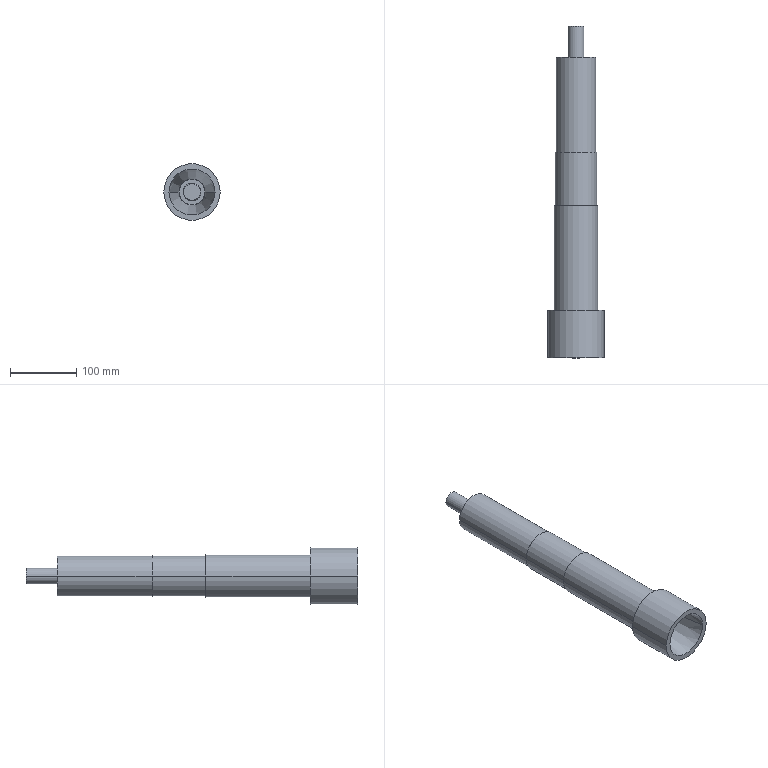Part | SolidWorks | features BaseBody 1 | 1 solid | 26 faces | box 85 x 500 x 85 mm | volume 1357723 mm3 | cylinder 12 | plane 8 | cone 4 | torus 2 | commonest cylinder face diameters 24 x2 25 x2 60 x2 62 x2 65 x2 85 x2
STEP:
#1=CARTESIAN_POINT('',(-2090.45,726.569,-1577.624));
#2=VERTEX_POINT('',#1);
#3=CARTESIAN_POINT('',(-2090.45,654.569,-1577.624));
#4=VERTEX_POINT('',#3);
#5=CARTESIAN_POINT('',(-2090.45,726.569,-1577.624));
#6=DIRECTION('',(0.,-1.,0.));
#7=VECTOR('',#6,1000.);
#8=LINE('',#5,#7);
#9=EDGE_CURVE('',#2,#4,#8,.T.);
#10=ORIENTED_EDGE('',*,*,#9,.F.);
#11=CARTESIAN_POINT('',(-2175.45,726.569,-1577.624));
#12=VERTEX_POINT('',#11);
#13=CARTESIAN_POINT('',(-2132.95,726.569,-1577.624));
#14=DIRECTION('',(0.,-1.,0.));
#15=DIRECTION('',(1.,0.,0.));
#16=AXIS2_PLACEMENT_3D('',#13,#14,#15);
#17=CIRCLE('',#16,42.5);
#18=EDGE_CURVE('',#2,#12,#17,.T.);
#19=ORIENTED_EDGE('',*,*,#18,.T.);
#20=CARTESIAN_POINT('',(-2175.45,654.569,-1577.624));
#21=VERTEX_POINT('',#20);
#22=CARTESIAN_POINT('',(-2175.45,726.569,-1577.624));
#23=DIRECTION('',(0.,-1.,0.));
#24=VECTOR('',#23,1000.);
#25=LINE('',#22,#24);
#26=EDGE_CURVE('',#12,#21,#25,.T.);
#27=ORIENTED_EDGE('',*,*,#26,.T.);
#28=CARTESIAN_POINT('',(-2132.95,654.569,-1577.624));
#29=DIRECTION('',(0.,-1.,0.));
#30=DIRECTION('',(1.,0.,0.));
#31=AXIS2_PLACEMENT_3D('',#28,#29,#30);
#32=CIRCLE('',#31,42.5);
#33=EDGE_CURVE('',#4,#21,#32,.T.);
#34=ORIENTED_EDGE('',*,*,#33,.F.);
#35=EDGE_LOOP('',(#10,#19,#27,#34));
#36=FACE_OUTER_BOUND('',#35,.T.);
#37=CARTESIAN_POINT('',(-2132.95,1154.569,-1577.624));
#38=DIRECTION('',(0.,1.,0.));
#39=DIRECTION('',(-1.,0.,0.));
#40=AXIS2_PLACEMENT_3D('',#37,#38,#39);
#41=CYLINDRICAL_SURFACE('',#40,42.5);
#42=ADVANCED_FACE('',(#36),#41,.T.);
#43=CARTESIAN_POINT('',(-2098.229,654.569,-1577.624));
#44=VERTEX_POINT('',#43);
#45=CARTESIAN_POINT('',(-2167.671,654.569,-1577.624));
#46=VERTEX_POINT('',#45);
#47=CARTESIAN_POINT('',(-2132.95,654.569,-1577.624));
#48=DIRECTION('',(0.,-1.,0.));
#49=DIRECTION('',(1.,0.,0.));
#50=AXIS2_PLACEMENT_3D('',#47,#48,#49);
#51=CIRCLE('',#50,34.721);
#52=EDGE_CURVE('',#44,#46,#51,.T.);
#53=ORIENTED_EDGE('',*,*,#52,.F.);
#54=CARTESIAN_POINT('',(-2132.95,654.569,-1577.624));
#55=DIRECTION('',(0.,-1.,0.));
#56=DIRECTION('',(-1.,0.,0.));
#57=AXIS2_PLACEMENT_3D('',#54,#55,#56);
#58=CIRCLE('',#57,34.721);
#59=EDGE_CURVE('',#46,#44,#58,.T.);
#60=ORIENTED_EDGE('',*,*,#59,.F.);
#61=EDGE_LOOP('',(#53,#60));
#62=FACE_BOUND('',#61,.T.);
#63=ORIENTED_EDGE('',*,*,#33,.T.);
#64=CARTESIAN_POINT('',(-2132.95,654.569,-1577.624));
#65=DIRECTION('',(0.,-1.,0.));
#66=DIRECTION('',(-1.,0.,0.));
#67=AXIS2_PLACEMENT_3D('',#64,#65,#66);
#68=CIRCLE('',#67,42.5);
#69=EDGE_CURVE('',#21,#4,#68,.T.);
#70=ORIENTED_EDGE('',*,*,#69,.T.);
#71=EDGE_LOOP('',(#63,#70));
#72=FACE_OUTER_BOUND('',#71,.T.);
#73=CARTESIAN_POINT('',(-2176.3,654.569,-1534.274));
#74=DIRECTION('',(0.,-1.,0.));
#75=DIRECTION('',(0.,0.,-1.));
#76=AXIS2_PLACEMENT_3D('',#73,#74,#75);
#77=PLANE('',#76);
#78=ADVANCED_FACE('',(#62,#72),#77,.T.);
#79=ORIENTED_EDGE('',*,*,#26,.F.);
#80=CARTESIAN_POINT('',(-2132.95,726.569,-1577.624));
#81=DIRECTION('',(0.,-1.,0.));
#82=DIRECTION('',(-1.,0.,0.));
#83=AXIS2_PLACEMENT_3D('',#80,#81,#82);
#84=CIRCLE('',#83,42.5);
#85=EDGE_CURVE('',#12,#2,#84,.T.);
#86=ORIENTED_EDGE('',*,*,#85,.T.);
#87=ORIENTED_EDGE('',*,*,#9,.T.);
#88=ORIENTED_EDGE('',*,*,#69,.F.);
#89=EDGE_LOOP('',(#79,#86,#87,#88));
#90=FACE_OUTER_BOUND('',#89,.T.);
#91=CARTESIAN_POINT('',(-2132.95,1154.569,-1577.624));
#92=DIRECTION('',(0.,1.,0.));
#93=DIRECTION('',(1.,0.,0.));
#94=AXIS2_PLACEMENT_3D('',#91,#92,#93);
#95=CYLINDRICAL_SURFACE('',#94,42.5);
#96=ADVANCED_FACE('',(#90),#95,.T.);
#97=CARTESIAN_POINT('',(-2144.95,1154.569,-1577.624));
#98=VERTEX_POINT('',#97);
#99=CARTESIAN_POINT('',(-2120.95,1154.569,-1577.624));
#100=VERTEX_POINT('',#99);
#101=CARTESIAN_POINT('',(-2132.95,1154.569,-1577.624));
#102=DIRECTION('',(0.,1.,0.));
#103=DIRECTION('',(-1.,0.,0.));
#104=AXIS2_PLACEMENT_3D('',#101,#102,#103);
#105=CIRCLE('',#104,12.);
#106=EDGE_CURVE('',#98,#100,#105,.T.);
#107=ORIENTED_EDGE('',*,*,#106,.T.);
#108=CARTESIAN_POINT('',(-2132.95,1154.569,-1577.624));
#109=DIRECTION('',(0.,1.,0.));
#110=DIRECTION('',(1.,0.,0.));
#111=AXIS2_PLACEMENT_3D('',#108,#109,#110);
#112=CIRCLE('',#111,12.);
#113=EDGE_CURVE('',#100,#98,#112,.T.);
#114=ORIENTED_EDGE('',*,*,#113,.T.);
#115=EDGE_LOOP('',(#107,#114));
#116=FACE_OUTER_BOUND('',#115,.T.);
#117=CARTESIAN_POINT('',(-2175.45,1154.569,-1620.124));
#118=DIRECTION('',(0.,1.,0.));
#119=DIRECTION('',(1.,0.,0.));
#120=AXIS2_PLACEMENT_3D('',#117,#118,#119);
#121=PLANE('',#120);
#122=ADVANCED_FACE('',(#116),#121,.T.);
#123=CARTESIAN_POINT('',(-2145.45,753.204,-1577.624));
#124=VERTEX_POINT('',#123);
#125=CARTESIAN_POINT('',(-2120.45,753.204,-1577.624));
#126=VERTEX_POINT('',#125);
#127=CARTESIAN_POINT('',(-2132.95,753.204,-1577.624));
#128=DIRECTION('',(0.,1.,0.));
#129=DIRECTION('',(-1.,0.,0.));
#130=AXIS2_PLACEMENT_3D('',#127,#128,#129);
#131=CIRCLE('',#130,12.5);
#132=EDGE_CURVE('',#124,#126,#131,.T.);
#133=ORIENTED_EDGE('',*,*,#132,.T.);
#134=CARTESIAN_POINT('',(-2119.431,754.969,-1577.624));
#135=VERTEX_POINT('',#134);
#136=CARTESIAN_POINT('',(-2119.431,754.969,-1577.624));
#137=DIRECTION('',(-0.5,-0.866,0.));
#138=VECTOR('',#137,1000.);
#139=LINE('',#136,#138);
#140=EDGE_CURVE('',#135,#126,#139,.T.);
#141=ORIENTED_EDGE('',*,*,#140,.F.);
#142=CARTESIAN_POINT('',(-2132.95,754.969,-1591.143));
#143=VERTEX_POINT('',#142);
#144=CARTESIAN_POINT('',(-2132.95,754.969,-1577.624));
#145=DIRECTION('',(0.,1.,0.));
#146=DIRECTION('',(0.,0.,-1.));
#147=AXIS2_PLACEMENT_3D('',#144,#145,#146);
#148=CIRCLE('',#147,13.519);
#149=EDGE_CURVE('',#143,#135,#148,.T.);
#150=ORIENTED_EDGE('',*,*,#149,.F.);
#151=CARTESIAN_POINT('',(-2132.95,753.204,-1590.124));
#152=VERTEX_POINT('',#151);
#153=CARTESIAN_POINT('',(-2132.95,753.204,-1590.124));
#154=DIRECTION('',(0.,0.866,-0.5));
#155=VECTOR('',#154,1000.);
#156=LINE('',#153,#155);
#157=EDGE_CURVE('',#152,#143,#156,.T.);
#158=ORIENTED_EDGE('',*,*,#157,.F.);
#159=CARTESIAN_POINT('',(-2132.95,753.204,-1577.624));
#160=DIRECTION('',(0.,1.,0.));
#161=DIRECTION('',(0.,0.,-1.));
#162=AXIS2_PLACEMENT_3D('',#159,#160,#161);
#163=CIRCLE('',#162,12.5);
#164=EDGE_CURVE('',#152,#124,#163,.T.);
#165=ORIENTED_EDGE('',*,*,#164,.T.);
#166=EDGE_LOOP('',(#133,#141,#150,#158,#165));
#167=FACE_OUTER_BOUND('',#166,.T.);
#168=CARTESIAN_POINT('',(-2132.95,753.116,-1577.624));
#169=DIRECTION('',(0.,1.,0.));
#170=DIRECTION('',(0.9962,0.,-0.08716));
#171=AXIS2_PLACEMENT_3D('',#168,#169,#170);
#172=CONICAL_SURFACE('',#171,12.449,0.5236);
#173=ADVANCED_FACE('',(#167),#172,.T.);
#174=CARTESIAN_POINT('',(-2153.153,754.113,-1577.624));
#175=VERTEX_POINT('',#174);
#176=CARTESIAN_POINT('',(-2167.671,654.569,-1577.624));
#177=DIRECTION('',(0.1443,0.9895,0.));
#178=VECTOR('',#177,1000.);
#179=LINE('',#176,#178);
#180=EDGE_CURVE('',#46,#175,#179,.T.);
#181=ORIENTED_EDGE('',*,*,#180,.F.);
#182=ORIENTED_EDGE('',*,*,#59,.T.);
#183=CARTESIAN_POINT('',(-2112.747,754.113,-1577.624));
#184=VERTEX_POINT('',#183);
#185=CARTESIAN_POINT('',(-2112.747,754.113,-1577.624));
#186=DIRECTION('',(0.1443,-0.9895,0.));
#187=VECTOR('',#186,1000.);
#188=LINE('',#185,#187);
#189=EDGE_CURVE('',#184,#44,#188,.T.);
#190=ORIENTED_EDGE('',*,*,#189,.F.);
#191=CARTESIAN_POINT('',(-2132.95,754.113,-1577.624));
#192=DIRECTION('',(0.,-1.,0.));
#193=DIRECTION('',(-1.,0.,0.));
#194=AXIS2_PLACEMENT_3D('',#191,#192,#193);
#195=CIRCLE('',#194,20.203);
#196=EDGE_CURVE('',#175,#184,#195,.T.);
#197=ORIENTED_EDGE('',*,*,#196,.F.);
#198=EDGE_LOOP('',(#181,#182,#190,#197));
#199=FACE_OUTER_BOUND('',#198,.T.);
#200=CARTESIAN_POINT('',(-2132.95,759.175,-1577.624));
#201=DIRECTION('',(0.,-1.,0.));
#202=DIRECTION('',(-0.9962,0.,0.08716));
#203=AXIS2_PLACEMENT_3D('',#200,#201,#202);
#204=CONICAL_SURFACE('',#203,19.465,0.1448);
#205=ADVANCED_FACE('',(#199),#204,.F.);
#206=CARTESIAN_POINT('',(-2132.95,754.113,-1577.624));
#207=DIRECTION('',(0.,-1.,0.));
#208=DIRECTION('',(0.,0.,1.));
#209=AXIS2_PLACEMENT_3D('',#206,#207,#208);
#210=CIRCLE('',#209,20.203);
#211=EDGE_CURVE('',#184,#175,#210,.T.);
#212=ORIENTED_EDGE('',*,*,#211,.T.);
#213=CARTESIAN_POINT('',(-2152.163,754.969,-1577.624));
#214=VERTEX_POINT('',#213);
#215=CARTESIAN_POINT('',(-2152.163,753.969,-1577.624));
#216=DIRECTION('',(0.,0.,1.));
#217=DIRECTION('',(0.,1.,0.));
#218=AXIS2_PLACEMENT_3D('',#215,#216,#217);
#219=CIRCLE('',#218,1.);
#220=EDGE_CURVE('',#214,#175,#219,.T.);
#221=ORIENTED_EDGE('',*,*,#220,.F.);
#222=CARTESIAN_POINT('',(-2113.736,754.969,-1577.624));
#223=VERTEX_POINT('',#222);
#224=CARTESIAN_POINT('',(-2132.95,754.969,-1577.624));
#225=DIRECTION('',(0.,1.,0.));
#226=DIRECTION('',(-1.,0.,0.));
#227=AXIS2_PLACEMENT_3D('',#224,#225,#226);
#228=CIRCLE('',#227,19.214);
#229=EDGE_CURVE('',#214,#223,#228,.T.);
#230=ORIENTED_EDGE('',*,*,#229,.T.);
#231=CARTESIAN_POINT('',(-2113.736,753.969,-1577.624));
#232=DIRECTION('',(0.,0.,1.));
#233=DIRECTION('',(0.9895,0.1443,0.));
#234=AXIS2_PLACEMENT_3D('',#231,#232,#233);
#235=CIRCLE('',#234,1.);
#236=EDGE_CURVE('',#184,#223,#235,.T.);
#237=ORIENTED_EDGE('',*,*,#236,.F.);
#238=EDGE_LOOP('',(#212,#221,#230,#237));
#239=FACE_OUTER_BOUND('',#238,.T.);
#240=CARTESIAN_POINT('',(-2132.95,753.969,-1577.624));
#241=DIRECTION('',(0.,1.,0.));
#242=DIRECTION('',(-0.9962,0.,-0.08716));
#243=AXIS2_PLACEMENT_3D('',#240,#241,#242);
#244=TOROIDAL_SURFACE('',#243,19.214,1.);
#245=ADVANCED_FACE('',(#239),#244,.F.);
#246=ORIENTED_EDGE('',*,*,#157,.T.);
#247=CARTESIAN_POINT('',(-2132.95,754.969,-1577.624));
#248=DIRECTION('',(0.,1.,0.));
#249=DIRECTION('',(1.,0.,0.));
#250=AXIS2_PLACEMENT_3D('',#247,#248,#249);
#251=CIRCLE('',#250,13.519);
#252=EDGE_CURVE('',#135,#143,#251,.T.);
#253=ORIENTED_EDGE('',*,*,#252,.F.);
#254=ORIENTED_EDGE('',*,*,#140,.T.);
#255=CARTESIAN_POINT('',(-2132.95,753.204,-1577.624));
#256=DIRECTION('',(0.,1.,0.));
#257=DIRECTION('',(1.,0.,0.));
#258=AXIS2_PLACEMENT_3D('',#255,#256,#257);
#259=CIRCLE('',#258,12.5);
#260=EDGE_CURVE('',#126,#152,#259,.T.);
#261=ORIENTED_EDGE('',*,*,#260,.T.);
#262=EDGE_LOOP('',(#246,#253,#254,#261));
#263=FACE_OUTER_BOUND('',#262,.T.);
#264=CARTESIAN_POINT('',(-2132.95,753.116,-1577.624));
#265=DIRECTION('',(0.,1.,0.));
#266=DIRECTION('',(-0.08716,0.,-0.9962));
#267=AXIS2_PLACEMENT_3D('',#264,#265,#266);
#268=CONICAL_SURFACE('',#267,12.449,0.5236);
#269=ADVANCED_FACE('',(#263),#268,.T.);
#270=ORIENTED_EDGE('',*,*,#211,.F.);
#271=ORIENTED_EDGE('',*,*,#189,.T.);
#272=ORIENTED_EDGE('',*,*,#52,.T.);
#273=ORIENTED_EDGE('',*,*,#180,.T.);
#274=EDGE_LOOP('',(#270,#271,#272,#273));
#275=FACE_OUTER_BOUND('',#274,.T.);
#276=CARTESIAN_POINT('',(-2132.95,759.175,-1577.624));
#277=DIRECTION('',(0.,-1.,0.));
#278=DIRECTION('',(0.9962,0.,-0.08716));
#279=AXIS2_PLACEMENT_3D('',#276,#277,#278);
#280=CONICAL_SURFACE('',#279,19.465,0.1448);
#281=ADVANCED_FACE('',(#275),#280,.F.);
#282=ORIENTED_EDGE('',*,*,#236,.T.);
#283=CARTESIAN_POINT('',(-2132.95,754.969,-1577.624));
#284=DIRECTION('',(0.,1.,0.));
#285=DIRECTION('',(1.,0.,0.));
#286=AXIS2_PLACEMENT_3D('',#283,#284,#285);
#287=CIRCLE('',#286,19.214);
#288=EDGE_CURVE('',#223,#214,#287,.T.);
#289=ORIENTED_EDGE('',*,*,#288,.T.);
#290=ORIENTED_EDGE('',*,*,#220,.T.);
#291=ORIENTED_EDGE('',*,*,#196,.T.);
#292=EDGE_LOOP('',(#282,#289,#290,#291));
#293=FACE_OUTER_BOUND('',#292,.T.);
#294=CARTESIAN_POINT('',(-2132.95,753.969,-1577.624));
#295=DIRECTION('',(0.,1.,0.));
#296=DIRECTION('',(0.9962,0.,0.08716));
#297=AXIS2_PLACEMENT_3D('',#294,#295,#296);
#298=TOROIDAL_SURFACE('',#297,19.214,1.);
#299=ADVANCED_FACE('',(#293),#298,.F.);
#300=ORIENTED_EDGE('',*,*,#252,.T.);
#301=ORIENTED_EDGE('',*,*,#149,.T.);
#302=EDGE_LOOP('',(#300,#301));
#303=FACE_BOUND('',#302,.T.);
#304=ORIENTED_EDGE('',*,*,#229,.F.);
#305=ORIENTED_EDGE('',*,*,#288,.F.);
#306=EDGE_LOOP('',(#304,#305));
#307=FACE_OUTER_BOUND('',#306,.T.);
#308=CARTESIAN_POINT('',(-2154.074,754.969,-1598.719));
#309=DIRECTION('',(0.,-1.,0.));
#310=DIRECTION('',(0.,0.,-1.));
#311=AXIS2_PLACEMENT_3D('',#308,#309,#310);
#312=PLANE('',#311);
#313=ADVANCED_FACE('',(#303,#307),#312,.T.);
#314=CARTESIAN_POINT('',(-2145.45,754.169,-1577.624));
#315=VERTEX_POINT('',#314);
#316=CARTESIAN_POINT('',(-2120.45,754.169,-1577.624));
#317=VERTEX_POINT('',#316);
#318=CARTESIAN_POINT('',(-2132.95,754.169,-1577.624));
#319=DIRECTION('',(0.,1.,0.));
#320=DIRECTION('',(-1.,0.,0.));
#321=AXIS2_PLACEMENT_3D('',#318,#319,#320);
#322=CIRCLE('',#321,12.5);
#323=EDGE_CURVE('',#315,#317,#322,.T.);
#324=ORIENTED_EDGE('',*,*,#323,.T.);
#325=CARTESIAN_POINT('',(-2120.45,754.169,-1577.624));
#326=DIRECTION('',(0.,-1.,0.));
#327=VECTOR('',#326,1000.);
#328=LINE('',#325,#327);
#329=EDGE_CURVE('',#317,#126,#328,.T.);
#330=ORIENTED_EDGE('',*,*,#329,.T.);
#331=ORIENTED_EDGE('',*,*,#132,.F.);
#332=CARTESIAN_POINT('',(-2145.45,754.169,-1577.624));
#333=DIRECTION('',(0.,-1.,0.));
#334=VECTOR('',#333,1000.);
#335=LINE('',#332,#334);
#336=EDGE_CURVE('',#315,#124,#335,.T.);
#337=ORIENTED_EDGE('',*,*,#336,.F.);
#338=EDGE_LOOP('',(#324,#330,#331,#337));
#339=FACE_OUTER_BOUND('',#338,.T.);
#340=CARTESIAN_POINT('',(-2132.95,754.169,-1577.624));
#341=DIRECTION('',(0.,1.,0.));
#342=DIRECTION('',(-1.,0.,0.));
#343=AXIS2_PLACEMENT_3D('',#340,#341,#342);
#344=CYLINDRICAL_SURFACE('',#343,12.5);
#345=ADVANCED_FACE('',(#339),#344,.F.);
#346=ORIENTED_EDGE('',*,*,#164,.F.);
#347=ORIENTED_EDGE('',*,*,#260,.F.);
#348=ORIENTED_EDGE('',*,*,#329,.F.);
#349=CARTESIAN_POINT('',(-2132.95,754.169,-1577.624));
#350=DIRECTION('',(0.,1.,0.));
#351=DIRECTION('',(1.,0.,0.));
#352=AXIS2_PLACEMENT_3D('',#349,#350,#351);
#353=CIRCLE('',#352,12.5);
#354=EDGE_CURVE('',#317,#315,#353,.T.);
#355=ORIENTED_EDGE('',*,*,#354,.T.);
#356=ORIENTED_EDGE('',*,*,#336,.T.);
#357=EDGE_LOOP('',(#346,#347,#348,#355,#356));
#358=FACE_OUTER_BOUND('',#357,.T.);
#359=CARTESIAN_POINT('',(-2132.95,754.169,-1577.624));
#360=DIRECTION('',(0.,1.,0.));
#361=DIRECTION('',(1.,0.,0.));
#362=AXIS2_PLACEMENT_3D('',#359,#360,#361);
#363=CYLINDRICAL_SURFACE('',#362,12.5);
#364=ADVANCED_FACE('',(#358),#363,.F.);
#365=ORIENTED_EDGE('',*,*,#323,.F.);
#366=ORIENTED_EDGE('',*,*,#354,.F.);
#367=EDGE_LOOP('',(#365,#366));
#368=FACE_OUTER_BOUND('',#367,.T.);
#369=CARTESIAN_POINT('',(-2145.7,754.169,-1590.374));
#370=DIRECTION('',(0.,-1.,0.));
#371=DIRECTION('',(0.,0.,-1.));
#372=AXIS2_PLACEMENT_3D('',#369,#370,#371);
#373=PLANE('',#372);
#374=ADVANCED_FACE('',(#368),#373,.T.);
#375=CARTESIAN_POINT('',(-2165.45,883.569,-1577.624));
#376=VERTEX_POINT('',#375);
#377=CARTESIAN_POINT('',(-2165.45,726.569,-1577.624));
#378=VERTEX_POINT('',#377);
#379=CARTESIAN_POINT('',(-2165.45,883.569,-1577.624));
#380=DIRECTION('',(0.,-1.,0.));
#381=VECTOR('',#380,1000.);
#382=LINE('',#379,#381);
#383=EDGE_CURVE('',#376,#378,#382,.T.);
#384=ORIENTED_EDGE('',*,*,#383,.F.);
#385=CARTESIAN_POINT('',(-2100.45,883.569,-1577.624));
#386=VERTEX_POINT('',#385);
#387=CARTESIAN_POINT('',(-2132.95,883.569,-1577.624));
#388=DIRECTION('',(0.,-1.,0.));
#389=DIRECTION('',(-1.,0.,0.));
#390=AXIS2_PLACEMENT_3D('',#387,#388,#389);
#391=CIRCLE('',#390,32.5);
#392=EDGE_CURVE('',#376,#386,#391,.T.);
#393=ORIENTED_EDGE('',*,*,#392,.T.);
#394=CARTESIAN_POINT('',(-2100.45,726.569,-1577.624));
#395=VERTEX_POINT('',#394);
#396=CARTESIAN_POINT('',(-2100.45,883.569,-1577.624));
#397=DIRECTION('',(0.,-1.,0.));
#398=VECTOR('',#397,1000.);
#399=LINE('',#396,#398);
#400=EDGE_CURVE('',#386,#395,#399,.T.);
#401=ORIENTED_EDGE('',*,*,#400,.T.);
#402=CARTESIAN_POINT('',(-2132.95,726.569,-1577.624));
#403=DIRECTION('',(0.,-1.,0.));
#404=DIRECTION('',(-1.,0.,0.));
#405=AXIS2_PLACEMENT_3D('',#402,#403,#404);
#406=CIRCLE('',#405,32.5);
#407=EDGE_CURVE('',#378,#395,#406,.T.);
#408=ORIENTED_EDGE('',*,*,#407,.F.);
#409=EDGE_LOOP('',(#384,#393,#401,#408));
#410=FACE_OUTER_BOUND('',#409,.T.);
#411=CARTESIAN_POINT('',(-2132.95,926.569,-1577.624));
#412=DIRECTION('',(0.,1.,0.));
#413=DIRECTION('',(1.,0.,0.));
#414=AXIS2_PLACEMENT_3D('',#411,#412,#413);
#415=CYLINDRICAL_SURFACE('',#414,32.5);
#416=ADVANCED_FACE('',(#410),#415,.T.);
#417=ORIENTED_EDGE('',*,*,#407,.T.);
#418=CARTESIAN_POINT('',(-2132.95,726.569,-1577.624));
#419=DIRECTION('',(0.,-1.,0.));
#420=DIRECTION('',(1.,0.,0.));
#421=AXIS2_PLACEMENT_3D('',#418,#419,#420);
#422=CIRCLE('',#421,32.5);
#423=EDGE_CURVE('',#395,#378,#422,.T.);
#424=ORIENTED_EDGE('',*,*,#423,.T.);
#425=EDGE_LOOP('',(#417,#424));
#426=FACE_BOUND('',#425,.T.);
#427=ORIENTED_EDGE('',*,*,#85,.F.);
#428=ORIENTED_EDGE('',*,*,#18,.F.);
#429=EDGE_LOOP('',(#427,#428));
#430=FACE_OUTER_BOUND('',#429,.T.);
#431=CARTESIAN_POINT('',(-2082.95,726.569,-1627.624));
#432=DIRECTION('',(0.,1.,0.));
#433=DIRECTION('',(1.,0.,0.));
#434=AXIS2_PLACEMENT_3D('',#431,#432,#433);
#435=PLANE('',#434);
#436=ADVANCED_FACE('',(#426,#430),#435,.T.);
#437=CARTESIAN_POINT('',(-2132.95,883.569,-1577.624));
#438=DIRECTION('',(0.,-1.,0.));
#439=DIRECTION('',(1.,0.,0.));
#440=AXIS2_PLACEMENT_3D('',#437,#438,#439);
#441=CIRCLE('',#440,32.5);
#442=EDGE_CURVE('',#386,#376,#441,.T.);
#443=ORIENTED_EDGE('',*,*,#442,.T.);
#444=ORIENTED_EDGE('',*,*,#383,.T.);
#445=ORIENTED_EDGE('',*,*,#423,.F.);
#446=ORIENTED_EDGE('',*,*,#400,.F.);
#447=EDGE_LOOP('',(#443,#444,#445,#446));
#448=FACE_OUTER_BOUND('',#447,.T.);
#449=CARTESIAN_POINT('',(-2132.95,926.569,-1577.624));
#450=DIRECTION('',(0.,1.,0.));
#451=DIRECTION('',(-1.,0.,0.));
#452=AXIS2_PLACEMENT_3D('',#449,#450,#451);
#453=CYLINDRICAL_SURFACE('',#452,32.5);
#454=ADVANCED_FACE('',(#448),#453,.T.);
#455=CARTESIAN_POINT('',(-2163.95,964.569,-1577.624));
#456=VERTEX_POINT('',#455);
#457=CARTESIAN_POINT('',(-2163.95,883.569,-1577.624));
#458=VERTEX_POINT('',#457);
#459=CARTESIAN_POINT('',(-2163.95,964.569,-1577.624));
#460=DIRECTION('',(0.,-1.,0.));
#461=VECTOR('',#460,1000.);
#462=LINE('',#459,#461);
#463=EDGE_CURVE('',#456,#458,#462,.T.);
#464=ORIENTED_EDGE('',*,*,#463,.F.);
#465=CARTESIAN_POINT('',(-2101.95,964.569,-1577.624));
#466=VERTEX_POINT('',#465);
#467=CARTESIAN_POINT('',(-2132.95,964.569,-1577.624));
#468=DIRECTION('',(0.,-1.,0.));
#469=DIRECTION('',(-1.,0.,0.));
#470=AXIS2_PLACEMENT_3D('',#467,#468,#469);
#471=CIRCLE('',#470,31.);
#472=EDGE_CURVE('',#456,#466,#471,.T.);
#473=ORIENTED_EDGE('',*,*,#472,.T.);
#474=CARTESIAN_POINT('',(-2101.95,883.569,-1577.624));
#475=VERTEX_POINT('',#474);
#476=CARTESIAN_POINT('',(-2101.95,964.569,-1577.624));
#477=DIRECTION('',(0.,-1.,0.));
#478=VECTOR('',#477,1000.);
#479=LINE('',#476,#478);
#480=EDGE_CURVE('',#466,#475,#479,.T.);
#481=ORIENTED_EDGE('',*,*,#480,.T.);
#482=CARTESIAN_POINT('',(-2132.95,883.569,-1577.624));
#483=DIRECTION('',(0.,-1.,0.));
#484=DIRECTION('',(-1.,0.,0.));
#485=AXIS2_PLACEMENT_3D('',#482,#483,#484);
#486=CIRCLE('',#485,31.);
#487=EDGE_CURVE('',#458,#475,#486,.T.);
#488=ORIENTED_EDGE('',*,*,#487,.F.);
#489=EDGE_LOOP('',(#464,#473,#481,#488));
#490=FACE_OUTER_BOUND('',#489,.T.);
#491=CARTESIAN_POINT('',(-2132.95,1083.569,-1577.624));
#492=DIRECTION('',(0.,1.,0.));
#493=DIRECTION('',(1.,0.,0.));
#494=AXIS2_PLACEMENT_3D('',#491,#492,#493);
#495=CYLINDRICAL_SURFACE('',#494,31.);
#496=ADVANCED_FACE('',(#490),#495,.T.);
#497=ORIENTED_EDGE('',*,*,#487,.T.);
#498=CARTESIAN_POINT('',(-2132.95,883.569,-1577.624));
#499=DIRECTION('',(0.,-1.,0.));
#500=DIRECTION('',(1.,0.,0.));
#501=AXIS2_PLACEMENT_3D('',#498,#499,#500);
#502=CIRCLE('',#501,31.);
#503=EDGE_CURVE('',#475,#458,#502,.T.);
#504=ORIENTED_EDGE('',*,*,#503,.T.);
#505=EDGE_LOOP('',(#497,#504));
#506=FACE_BOUND('',#505,.T.);
#507=ORIENTED_EDGE('',*,*,#442,.F.);
#508=ORIENTED_EDGE('',*,*,#392,.F.);
#509=EDGE_LOOP('',(#507,#508));
#510=FACE_OUTER_BOUND('',#509,.T.);
#511=CARTESIAN_POINT('',(-2082.95,883.569,-1627.624));
#512=DIRECTION('',(0.,1.,0.));
#513=DIRECTION('',(1.,0.,0.));
#514=AXIS2_PLACEMENT_3D('',#511,#512,#513);
#515=PLANE('',#514);
#516=ADVANCED_FACE('',(#506,#510),#515,.T.);
#517=CARTESIAN_POINT('',(-2132.95,964.569,-1577.624));
#518=DIRECTION('',(0.,-1.,0.));
#519=DIRECTION('',(1.,0.,0.));
#520=AXIS2_PLACEMENT_3D('',#517,#518,#519);
#521=CIRCLE('',#520,31.);
#522=EDGE_CURVE('',#466,#456,#521,.T.);
#523=ORIENTED_EDGE('',*,*,#522,.T.);
#524=ORIENTED_EDGE('',*,*,#463,.T.);
#525=ORIENTED_EDGE('',*,*,#503,.F.);
#526=ORIENTED_EDGE('',*,*,#480,.F.);
#527=EDGE_LOOP('',(#523,#524,#525,#526));
#528=FACE_OUTER_BOUND('',#527,.T.);
#529=CARTESIAN_POINT('',(-2132.95,1083.569,-1577.624));
#530=DIRECTION('',(0.,1.,0.));
#531=DIRECTION('',(-1.,0.,0.));
#532=AXIS2_PLACEMENT_3D('',#529,#530,#531);
#533=CYLINDRICAL_SURFACE('',#532,31.);
#534=ADVANCED_FACE('',(#528),#533,.T.);
#535=CARTESIAN_POINT('',(-2162.95,1107.569,-1577.624));
#536=VERTEX_POINT('',#535);
#537=CARTESIAN_POINT('',(-2162.95,964.569,-1577.624));
#538=VERTEX_POINT('',#537);
#539=CARTESIAN_POINT('',(-2162.95,1107.569,-1577.624));
#540=DIRECTION('',(0.,-1.,0.));
#541=VECTOR('',#540,1000.);
#542=LINE('',#539,#541);
#543=EDGE_CURVE('',#536,#538,#542,.T.);
#544=ORIENTED_EDGE('',*,*,#543,.F.);
#545=CARTESIAN_POINT('',(-2102.95,1107.569,-1577.624));
#546=VERTEX_POINT('',#545);
#547=CARTESIAN_POINT('',(-2132.95,1107.569,-1577.624));
#548=DIRECTION('',(0.,-1.,0.));
#549=DIRECTION('',(-1.,0.,0.));
#550=AXIS2_PLACEMENT_3D('',#547,#548,#549);
#551=CIRCLE('',#550,30.);
#552=EDGE_CURVE('',#536,#546,#551,.T.);
#553=ORIENTED_EDGE('',*,*,#552,.T.);
#554=CARTESIAN_POINT('',(-2102.95,964.569,-1577.624));
#555=VERTEX_POINT('',#554);
#556=CARTESIAN_POINT('',(-2102.95,1107.569,-1577.624));
#557=DIRECTION('',(0.,-1.,0.));
#558=VECTOR('',#557,1000.);
#559=LINE('',#556,#558);
#560=EDGE_CURVE('',#546,#555,#559,.T.);
#561=ORIENTED_EDGE('',*,*,#560,.T.);
#562=CARTESIAN_POINT('',(-2132.95,964.569,-1577.624));
#563=DIRECTION('',(0.,-1.,0.));
#564=DIRECTION('',(-1.,0.,0.));
#565=AXIS2_PLACEMENT_3D('',#562,#563,#564);
#566=CIRCLE('',#565,30.);
#567=EDGE_CURVE('',#538,#555,#566,.T.);
#568=ORIENTED_EDGE('',*,*,#567,.F.);
#569=EDGE_LOOP('',(#544,#553,#561,#568));
#570=FACE_OUTER_BOUND('',#569,.T.);
#571=CARTESIAN_POINT('',(-2132.95,1164.569,-1577.624));
#572=DIRECTION('',(0.,1.,0.));
#573=DIRECTION('',(1.,0.,0.));
#574=AXIS2_PLACEMENT_3D('',#571,#572,#573);
#575=CYLINDRICAL_SURFACE('',#574,30.);
#576=ADVANCED_FACE('',(#570),#575,.T.);
#577=ORIENTED_EDGE('',*,*,#567,.T.);
#578=CARTESIAN_POINT('',(-2132.95,964.569,-1577.624));
#579=DIRECTION('',(0.,-1.,0.));
#580=DIRECTION('',(1.,0.,0.));
#581=AXIS2_PLACEMENT_3D('',#578,#579,#580);
#582=CIRCLE('',#581,30.);
#583=EDGE_CURVE('',#555,#538,#582,.T.);
#584=ORIENTED_EDGE('',*,*,#583,.T.);
#585=EDGE_LOOP('',(#577,#584));
#586=FACE_BOUND('',#585,.T.);
#587=ORIENTED_EDGE('',*,*,#522,.F.);
#588=ORIENTED_EDGE('',*,*,#472,.F.);
#589=EDGE_LOOP('',(#587,#588));
#590=FACE_OUTER_BOUND('',#589,.T.);
#591=CARTESIAN_POINT('',(-2082.95,964.569,-1627.624));
#592=DIRECTION('',(0.,1.,0.));
#593=DIRECTION('',(1.,0.,0.));
#594=AXIS2_PLACEMENT_3D('',#591,#592,#593);
#595=PLANE('',#594);
#596=ADVANCED_FACE('',(#586,#590),#595,.T.);
#597=CARTESIAN_POINT('',(-2132.95,1107.569,-1577.624));
#598=DIRECTION('',(0.,-1.,0.));
#599=DIRECTION('',(1.,0.,0.));
#600=AXIS2_PLACEMENT_3D('',#597,#598,#599);
#601=CIRCLE('',#600,30.);
#602=EDGE_CURVE('',#546,#536,#601,.T.);
#603=ORIENTED_EDGE('',*,*,#602,.T.);
#604=ORIENTED_EDGE('',*,*,#543,.T.);
#605=ORIENTED_EDGE('',*,*,#583,.F.);
#606=ORIENTED_EDGE('',*,*,#560,.F.);
#607=EDGE_LOOP('',(#603,#604,#605,#606));
#608=FACE_OUTER_BOUND('',#607,.T.);
#609=CARTESIAN_POINT('',(-2132.95,1164.569,-1577.624));
#610=DIRECTION('',(0.,1.,0.));
#611=DIRECTION('',(-1.,0.,0.));
#612=AXIS2_PLACEMENT_3D('',#609,#610,#611);
#613=CYLINDRICAL_SURFACE('',#612,30.);
#614=ADVANCED_FACE('',(#608),#613,.T.);
#615=CARTESIAN_POINT('',(-2144.95,1107.569,-1577.624));
#616=VERTEX_POINT('',#615);
#617=CARTESIAN_POINT('',(-2144.95,1154.569,-1577.624));
#618=DIRECTION('',(0.,-1.,0.));
#619=VECTOR('',#618,1000.);
#620=LINE('',#617,#619);
#621=EDGE_CURVE('',#98,#616,#620,.T.);
#622=ORIENTED_EDGE('',*,*,#621,.F.);
#623=ORIENTED_EDGE('',*,*,#113,.F.);
#624=CARTESIAN_POINT('',(-2120.95,1107.569,-1577.624));
#625=VERTEX_POINT('',#624);
#626=CARTESIAN_POINT('',(-2120.95,1154.569,-1577.624));
#627=DIRECTION('',(0.,-1.,0.));
#628=VECTOR('',#627,1000.);
#629=LINE('',#626,#628);
#630=EDGE_CURVE('',#100,#625,#629,.T.);
#631=ORIENTED_EDGE('',*,*,#630,.T.);
#632=CARTESIAN_POINT('',(-2132.95,1107.569,-1577.624));
#633=DIRECTION('',(0.,-1.,0.));
#634=DIRECTION('',(-1.,0.,0.));
#635=AXIS2_PLACEMENT_3D('',#632,#633,#634);
#636=CIRCLE('',#635,12.);
#637=EDGE_CURVE('',#616,#625,#636,.T.);
#638=ORIENTED_EDGE('',*,*,#637,.F.);
#639=EDGE_LOOP('',(#622,#623,#631,#638));
#640=FACE_OUTER_BOUND('',#639,.T.);
#641=CARTESIAN_POINT('',(-2132.95,1307.569,-1577.624));
#642=DIRECTION('',(0.,1.,0.));
#643=DIRECTION('',(1.,0.,0.));
#644=AXIS2_PLACEMENT_3D('',#641,#642,#643);
#645=CYLINDRICAL_SURFACE('',#644,12.);
#646=ADVANCED_FACE('',(#640),#645,.T.);
#647=ORIENTED_EDGE('',*,*,#637,.T.);
#648=CARTESIAN_POINT('',(-2132.95,1107.569,-1577.624));
#649=DIRECTION('',(0.,-1.,0.));
#650=DIRECTION('',(1.,0.,0.));
#651=AXIS2_PLACEMENT_3D('',#648,#649,#650);
#652=CIRCLE('',#651,12.);
#653=EDGE_CURVE('',#625,#616,#652,.T.);
#654=ORIENTED_EDGE('',*,*,#653,.T.);
#655=EDGE_LOOP('',(#647,#654));
#656=FACE_BOUND('',#655,.T.);
#657=ORIENTED_EDGE('',*,*,#602,.F.);
#658=ORIENTED_EDGE('',*,*,#552,.F.);
#659=EDGE_LOOP('',(#657,#658));
#660=FACE_OUTER_BOUND('',#659,.T.);
#661=CARTESIAN_POINT('',(-2082.95,1107.569,-1627.624));
#662=DIRECTION('',(0.,1.,0.));
#663=DIRECTION('',(1.,0.,0.));
#664=AXIS2_PLACEMENT_3D('',#661,#662,#663);
#665=PLANE('',#664);
#666=ADVANCED_FACE('',(#656,#660),#665,.T.);
#667=ORIENTED_EDGE('',*,*,#106,.F.);
#668=ORIENTED_EDGE('',*,*,#621,.T.);
#669=ORIENTED_EDGE('',*,*,#653,.F.);
#670=ORIENTED_EDGE('',*,*,#630,.F.);
#671=EDGE_LOOP('',(#667,#668,#669,#670));
#672=FACE_OUTER_BOUND('',#671,.T.);
#673=CARTESIAN_POINT('',(-2132.95,1307.569,-1577.624));
#674=DIRECTION('',(0.,1.,0.));
#675=DIRECTION('',(-1.,0.,0.));
#676=AXIS2_PLACEMENT_3D('',#673,#674,#675);
#677=CYLINDRICAL_SURFACE('',#676,12.);
#678=ADVANCED_FACE('',(#672),#677,.T.);
#679=CLOSED_SHELL('',(#42,#78,#96,#122,#173,#205,#245,#269,#281,#299,#313,#345,#364,#374,#416,#436,#454,#496,#516,#534,#576,#596,#614,#646,#666,#678));
#680=MANIFOLD_SOLID_BREP('',#679);
#681=CARTESIAN_POINT('',(0.,0.,0.));
#682=DIRECTION('',(0.,0.,1.));
#683=DIRECTION('',(1.,0.,0.));
#684=AXIS2_PLACEMENT_3D('',#681,#682,#683);
#685=(LENGTH_UNIT()NAMED_UNIT(*)SI_UNIT(.MILLI.,.METRE.));
#686=UNCERTAINTY_MEASURE_WITH_UNIT(LENGTH_MEASURE(0.00001),#685,'','');
#687=(NAMED_UNIT(*)PLANE_ANGLE_UNIT()SI_UNIT($,.RADIAN.));
#688=(NAMED_UNIT(*)SI_UNIT($,.STERADIAN.)SOLID_ANGLE_UNIT());
#689=(GEOMETRIC_REPRESENTATION_CONTEXT(3)GLOBAL_UNCERTAINTY_ASSIGNED_CONTEXT((#686))GLOBAL_UNIT_ASSIGNED_CONTEXT((#685,#687,#688))REPRESENTATION_CONTEXT('',''));
#690=ADVANCED_BREP_SHAPE_REPRESENTATION('',(#680,#684),#689);